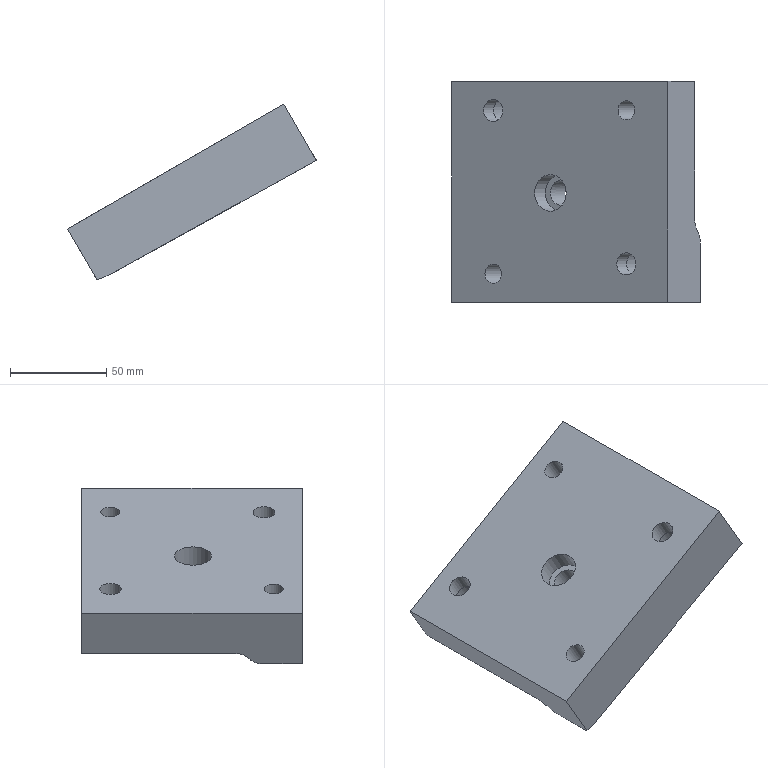Part | NX | features solid 2 | 1 solid | 30 faces | box 129.432 x 115 x 91.447 mm | volume 400610 mm3 | spline 15 | cylinder 8 | plane 7 | commonest cylinder face diameters 10 x2 11.5 x2 17.5 x2 13 x1 19 x1